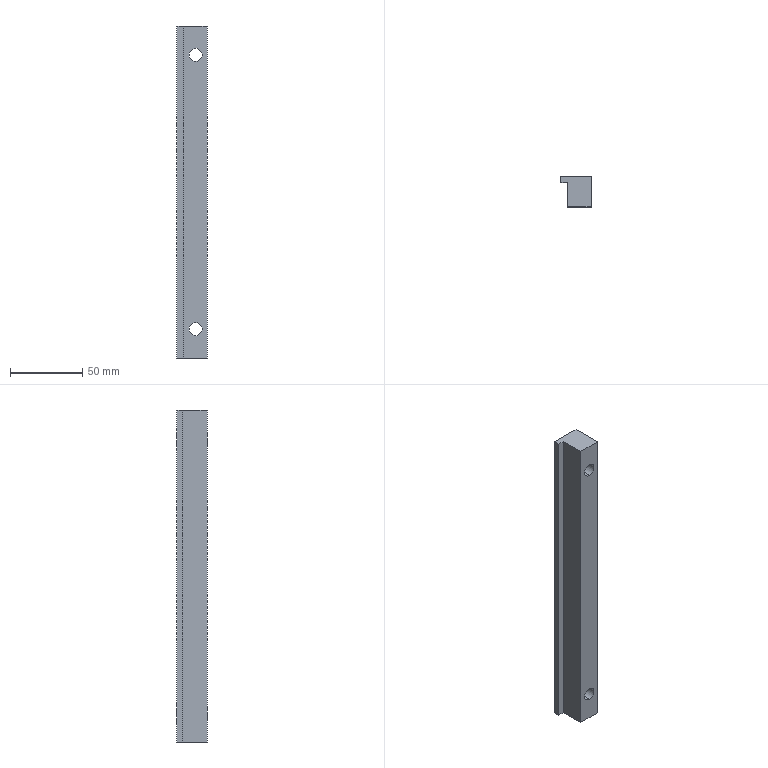Part | STEP file | LM-05-1197_default | 1 solid | 18 faces | box 21 x 21 x 230 mm | volume 79008 mm3 | plane 10 | cylinder 8 | commonest cylinder face diameters 9 x4 15 x4
STEP:
#1=CARTESIAN_POINT('',(0.,0.,0.));
#2=DIRECTION('',(0.,0.,1.));
#3=DIRECTION('',(1.,0.,0.));
#4=AXIS2_PLACEMENT_3D('',#1,#2,#3);
#5=CARTESIAN_POINT('',(13.,-8.6,217.5));
#6=VERTEX_POINT('',#5);
#7=CARTESIAN_POINT('',(13.,0.,217.5));
#8=VERTEX_POINT('',#7);
#9=CARTESIAN_POINT('',(13.,0.,217.5));
#10=DIRECTION('',(0.,1.,0.));
#11=VECTOR('',#10,1.);
#12=LINE('',#9,#11);
#13=CARTESIAN_POINT('',(13.,0.,210.));
#14=DIRECTION('',(0.,1.,0.));
#15=DIRECTION('',(0.,0.,1.));
#16=AXIS2_PLACEMENT_3D('',#13,#14,#15);
#17=CYLINDRICAL_SURFACE('',#16,7.5);
#18=CARTESIAN_POINT('',(6.283,0.));
#19=DIRECTION('',(0.,1.));
#20=VECTOR('',#19,1.);
#21=LINE('',#18,#20);
#22=(GEOMETRIC_REPRESENTATION_CONTEXT(2)PARAMETRIC_REPRESENTATION_CONTEXT()REPRESENTATION_CONTEXT('',''));
#23=DEFINITIONAL_REPRESENTATION('',(#21),#22);
#24=PCURVE('',#17,#23);
#25=CARTESIAN_POINT('',(13.,0.,210.));
#26=DIRECTION('',(0.,1.,0.));
#27=DIRECTION('',(0.,0.,1.));
#28=AXIS2_PLACEMENT_3D('',#25,#26,#27);
#29=CYLINDRICAL_SURFACE('',#28,7.5);
#30=CARTESIAN_POINT('',(0.,0.));
#31=DIRECTION('',(0.,1.));
#32=VECTOR('',#31,1.);
#33=LINE('',#30,#32);
#34=(GEOMETRIC_REPRESENTATION_CONTEXT(2)PARAMETRIC_REPRESENTATION_CONTEXT()REPRESENTATION_CONTEXT('',''));
#35=DEFINITIONAL_REPRESENTATION('',(#33),#34);
#36=PCURVE('',#29,#35);
#37=SURFACE_CURVE('',#12,(#24,#36),.PCURVE_S1.);
#38=EDGE_CURVE('',#6,#8,#37,.T.);
#39=ORIENTED_EDGE('',*,*,#38,.T.);
#40=CARTESIAN_POINT('',(13.,0.,202.5));
#41=VERTEX_POINT('',#40);
#42=CARTESIAN_POINT('',(13.,0.,210.));
#43=DIRECTION('',(0.,1.,0.));
#44=DIRECTION('',(0.,0.,1.));
#45=AXIS2_PLACEMENT_3D('',#42,#43,#44);
#46=CIRCLE('',#45,7.5);
#47=CARTESIAN_POINT('',(0.,0.));
#48=DIRECTION('',(1.,0.));
#49=VECTOR('',#48,1.);
#50=LINE('',#47,#49);
#51=(GEOMETRIC_REPRESENTATION_CONTEXT(2)PARAMETRIC_REPRESENTATION_CONTEXT()REPRESENTATION_CONTEXT('',''));
#52=DEFINITIONAL_REPRESENTATION('',(#50),#51);
#53=PCURVE('',#17,#52);
#54=CARTESIAN_POINT('',(21.,0.,230.));
#55=DIRECTION('',(0.,-1.,0.));
#56=DIRECTION('',(1.,0.,0.));
#57=AXIS2_PLACEMENT_3D('',#54,#55,#56);
#58=PLANE('',#57);
#59=CARTESIAN_POINT('',(-8.,-12.5));
#60=CARTESIAN_POINT('',(4.99,-12.5));
#61=CARTESIAN_POINT('',(-1.505,-23.75));
#62=CARTESIAN_POINT('',(-8.,-35.));
#63=CARTESIAN_POINT('',(-14.495,-23.75));
#64=CARTESIAN_POINT('',(-20.99,-12.5));
#65=CARTESIAN_POINT('',(-8.,-12.5));
#66=(BOUNDED_CURVE()B_SPLINE_CURVE(2,(#59,#60,#61,#62,#63,#64,#65),.UNSPECIFIED.,.T.,.F.)B_SPLINE_CURVE_WITH_KNOTS((1,2,2,2,2,1),(-2.094,0.,2.094,4.189,6.283,8.378),.UNSPECIFIED.)CURVE()GEOMETRIC_REPRESENTATION_ITEM()RATIONAL_B_SPLINE_CURVE((1.,0.5,1.,0.5,1.,0.5,1.))REPRESENTATION_ITEM(''));
#67=(GEOMETRIC_REPRESENTATION_CONTEXT(2)PARAMETRIC_REPRESENTATION_CONTEXT()REPRESENTATION_CONTEXT('',''));
#68=DEFINITIONAL_REPRESENTATION('',(#66),#67);
#69=PCURVE('',#58,#68);
#70=SURFACE_CURVE('',#46,(#53,#69),.PCURVE_S1.);
#71=EDGE_CURVE('',#41,#8,#70,.T.);
#72=ORIENTED_EDGE('',*,*,#71,.F.);
#73=CARTESIAN_POINT('',(13.,-8.6,202.5));
#74=VERTEX_POINT('',#73);
#75=CARTESIAN_POINT('',(13.,0.,202.5));
#76=DIRECTION('',(0.,1.,0.));
#77=VECTOR('',#76,1.);
#78=LINE('',#75,#77);
#79=CARTESIAN_POINT('',(3.142,0.));
#80=DIRECTION('',(0.,1.));
#81=VECTOR('',#80,1.);
#82=LINE('',#79,#81);
#83=(GEOMETRIC_REPRESENTATION_CONTEXT(2)PARAMETRIC_REPRESENTATION_CONTEXT()REPRESENTATION_CONTEXT('',''));
#84=DEFINITIONAL_REPRESENTATION('',(#82),#83);
#85=PCURVE('',#17,#84);
#86=CARTESIAN_POINT('',(3.142,0.));
#87=DIRECTION('',(0.,1.));
#88=VECTOR('',#87,1.);
#89=LINE('',#86,#88);
#90=(GEOMETRIC_REPRESENTATION_CONTEXT(2)PARAMETRIC_REPRESENTATION_CONTEXT()REPRESENTATION_CONTEXT('',''));
#91=DEFINITIONAL_REPRESENTATION('',(#89),#90);
#92=PCURVE('',#29,#91);
#93=SURFACE_CURVE('',#78,(#85,#92),.PCURVE_S1.);
#94=EDGE_CURVE('',#74,#41,#93,.T.);
#95=ORIENTED_EDGE('',*,*,#94,.F.);
#96=CARTESIAN_POINT('',(13.,-8.6,210.));
#97=DIRECTION('',(0.,1.,0.));
#98=DIRECTION('',(0.,0.,1.));
#99=AXIS2_PLACEMENT_3D('',#96,#97,#98);
#100=CIRCLE('',#99,7.5);
#101=CARTESIAN_POINT('',(0.,-8.6));
#102=DIRECTION('',(1.,0.));
#103=VECTOR('',#102,1.);
#104=LINE('',#101,#103);
#105=(GEOMETRIC_REPRESENTATION_CONTEXT(2)PARAMETRIC_REPRESENTATION_CONTEXT()REPRESENTATION_CONTEXT('',''));
#106=DEFINITIONAL_REPRESENTATION('',(#104),#105);
#107=PCURVE('',#17,#106);
#108=CARTESIAN_POINT('',(17.5,-8.6,210.));
#109=DIRECTION('',(0.,-1.,0.));
#110=DIRECTION('',(0.,0.,-1.));
#111=AXIS2_PLACEMENT_3D('',#108,#109,#110);
#112=PLANE('',#111);
#113=CARTESIAN_POINT('',(-7.5,-4.5));
#114=CARTESIAN_POINT('',(-7.5,8.49));
#115=CARTESIAN_POINT('',(3.75,1.995));
#116=CARTESIAN_POINT('',(15.,-4.5));
#117=CARTESIAN_POINT('',(3.75,-10.995));
#118=CARTESIAN_POINT('',(-7.5,-17.49));
#119=CARTESIAN_POINT('',(-7.5,-4.5));
#120=(BOUNDED_CURVE()B_SPLINE_CURVE(2,(#113,#114,#115,#116,#117,#118,#119),.UNSPECIFIED.,.T.,.F.)B_SPLINE_CURVE_WITH_KNOTS((1,2,2,2,2,1),(-2.094,0.,2.094,4.189,6.283,8.378),.UNSPECIFIED.)CURVE()GEOMETRIC_REPRESENTATION_ITEM()RATIONAL_B_SPLINE_CURVE((1.,0.5,1.,0.5,1.,0.5,1.))REPRESENTATION_ITEM(''));
#121=(GEOMETRIC_REPRESENTATION_CONTEXT(2)PARAMETRIC_REPRESENTATION_CONTEXT()REPRESENTATION_CONTEXT('',''));
#122=DEFINITIONAL_REPRESENTATION('',(#120),#121);
#123=PCURVE('',#112,#122);
#124=SURFACE_CURVE('',#100,(#107,#123),.PCURVE_S1.);
#125=EDGE_CURVE('',#74,#6,#124,.T.);
#126=ORIENTED_EDGE('',*,*,#125,.T.);
#127=EDGE_LOOP('',(#39,#72,#95,#126));
#128=FACE_BOUND('',#127,.F.);
#129=ADVANCED_FACE('',(#128),#17,.F.);
#130=CARTESIAN_POINT('',(13.,-21.,214.5));
#131=VERTEX_POINT('',#130);
#132=CARTESIAN_POINT('',(13.,-8.6,214.5));
#133=VERTEX_POINT('',#132);
#134=CARTESIAN_POINT('',(13.,0.,214.5));
#135=DIRECTION('',(0.,1.,0.));
#136=VECTOR('',#135,1.);
#137=LINE('',#134,#136);
#138=CARTESIAN_POINT('',(13.,0.,210.));
#139=DIRECTION('',(0.,1.,0.));
#140=DIRECTION('',(0.,0.,1.));
#141=AXIS2_PLACEMENT_3D('',#138,#139,#140);
#142=CYLINDRICAL_SURFACE('',#141,4.5);
#143=CARTESIAN_POINT('',(6.283,0.));
#144=DIRECTION('',(0.,1.));
#145=VECTOR('',#144,1.);
#146=LINE('',#143,#145);
#147=(GEOMETRIC_REPRESENTATION_CONTEXT(2)PARAMETRIC_REPRESENTATION_CONTEXT()REPRESENTATION_CONTEXT('',''));
#148=DEFINITIONAL_REPRESENTATION('',(#146),#147);
#149=PCURVE('',#142,#148);
#150=CARTESIAN_POINT('',(13.,0.,210.));
#151=DIRECTION('',(0.,1.,0.));
#152=DIRECTION('',(0.,0.,1.));
#153=AXIS2_PLACEMENT_3D('',#150,#151,#152);
#154=CYLINDRICAL_SURFACE('',#153,4.5);
#155=CARTESIAN_POINT('',(0.,0.));
#156=DIRECTION('',(0.,1.));
#157=VECTOR('',#156,1.);
#158=LINE('',#155,#157);
#159=(GEOMETRIC_REPRESENTATION_CONTEXT(2)PARAMETRIC_REPRESENTATION_CONTEXT()REPRESENTATION_CONTEXT('',''));
#160=DEFINITIONAL_REPRESENTATION('',(#158),#159);
#161=PCURVE('',#154,#160);
#162=SURFACE_CURVE('',#137,(#149,#161),.PCURVE_S1.);
#163=EDGE_CURVE('',#131,#133,#162,.T.);
#164=ORIENTED_EDGE('',*,*,#163,.T.);
#165=CARTESIAN_POINT('',(13.,-8.6,205.5));
#166=VERTEX_POINT('',#165);
#167=CARTESIAN_POINT('',(13.,-8.6,210.));
#168=DIRECTION('',(0.,1.,0.));
#169=DIRECTION('',(0.,0.,1.));
#170=AXIS2_PLACEMENT_3D('',#167,#168,#169);
#171=CIRCLE('',#170,4.5);
#172=CARTESIAN_POINT('',(0.,-8.6));
#173=DIRECTION('',(1.,0.));
#174=VECTOR('',#173,1.);
#175=LINE('',#172,#174);
#176=(GEOMETRIC_REPRESENTATION_CONTEXT(2)PARAMETRIC_REPRESENTATION_CONTEXT()REPRESENTATION_CONTEXT('',''));
#177=DEFINITIONAL_REPRESENTATION('',(#175),#176);
#178=PCURVE('',#142,#177);
#179=CARTESIAN_POINT('',(-4.5,-4.5));
#180=CARTESIAN_POINT('',(-4.5,3.294));
#181=CARTESIAN_POINT('',(2.25,-0.6029));
#182=CARTESIAN_POINT('',(9.,-4.5));
#183=CARTESIAN_POINT('',(2.25,-8.397));
#184=CARTESIAN_POINT('',(-4.5,-12.294));
#185=CARTESIAN_POINT('',(-4.5,-4.5));
#186=(BOUNDED_CURVE()B_SPLINE_CURVE(2,(#179,#180,#181,#182,#183,#184,#185),.UNSPECIFIED.,.T.,.F.)B_SPLINE_CURVE_WITH_KNOTS((1,2,2,2,2,1),(-2.094,0.,2.094,4.189,6.283,8.378),.UNSPECIFIED.)CURVE()GEOMETRIC_REPRESENTATION_ITEM()RATIONAL_B_SPLINE_CURVE((1.,0.5,1.,0.5,1.,0.5,1.))REPRESENTATION_ITEM(''));
#187=(GEOMETRIC_REPRESENTATION_CONTEXT(2)PARAMETRIC_REPRESENTATION_CONTEXT()REPRESENTATION_CONTEXT('',''));
#188=DEFINITIONAL_REPRESENTATION('',(#186),#187);
#189=PCURVE('',#112,#188);
#190=SURFACE_CURVE('',#171,(#178,#189),.PCURVE_S1.);
#191=EDGE_CURVE('',#166,#133,#190,.T.);
#192=ORIENTED_EDGE('',*,*,#191,.F.);
#193=CARTESIAN_POINT('',(13.,-21.,205.5));
#194=VERTEX_POINT('',#193);
#195=CARTESIAN_POINT('',(13.,0.,205.5));
#196=DIRECTION('',(0.,1.,0.));
#197=VECTOR('',#196,1.);
#198=LINE('',#195,#197);
#199=CARTESIAN_POINT('',(3.142,0.));
#200=DIRECTION('',(0.,1.));
#201=VECTOR('',#200,1.);
#202=LINE('',#199,#201);
#203=(GEOMETRIC_REPRESENTATION_CONTEXT(2)PARAMETRIC_REPRESENTATION_CONTEXT()REPRESENTATION_CONTEXT('',''));
#204=DEFINITIONAL_REPRESENTATION('',(#202),#203);
#205=PCURVE('',#142,#204);
#206=CARTESIAN_POINT('',(3.142,0.));
#207=DIRECTION('',(0.,1.));
#208=VECTOR('',#207,1.);
#209=LINE('',#206,#208);
#210=(GEOMETRIC_REPRESENTATION_CONTEXT(2)PARAMETRIC_REPRESENTATION_CONTEXT()REPRESENTATION_CONTEXT('',''));
#211=DEFINITIONAL_REPRESENTATION('',(#209),#210);
#212=PCURVE('',#154,#211);
#213=SURFACE_CURVE('',#198,(#205,#212),.PCURVE_S1.);
#214=EDGE_CURVE('',#194,#166,#213,.T.);
#215=ORIENTED_EDGE('',*,*,#214,.F.);
#216=CARTESIAN_POINT('',(13.,-21.,210.));
#217=DIRECTION('',(0.,1.,0.));
#218=DIRECTION('',(0.,0.,1.));
#219=AXIS2_PLACEMENT_3D('',#216,#217,#218);
#220=CIRCLE('',#219,4.5);
#221=CARTESIAN_POINT('',(0.,-21.));
#222=DIRECTION('',(1.,0.));
#223=VECTOR('',#222,1.);
#224=LINE('',#221,#223);
#225=(GEOMETRIC_REPRESENTATION_CONTEXT(2)PARAMETRIC_REPRESENTATION_CONTEXT()REPRESENTATION_CONTEXT('',''));
#226=DEFINITIONAL_REPRESENTATION('',(#224),#225);
#227=PCURVE('',#142,#226);
#228=CARTESIAN_POINT('',(4.554,-21.,230.));
#229=DIRECTION('',(0.,1.,0.));
#230=DIRECTION('',(0.,0.,1.));
#231=AXIS2_PLACEMENT_3D('',#228,#229,#230);
#232=PLANE('',#231);
#233=CARTESIAN_POINT('',(-20.,8.446));
#234=DIRECTION('',(1.,0.));
#235=AXIS2_PLACEMENT_2D('',#233,#234);
#236=CIRCLE('',#235,4.5);
#237=(GEOMETRIC_REPRESENTATION_CONTEXT(2)PARAMETRIC_REPRESENTATION_CONTEXT()REPRESENTATION_CONTEXT('',''));
#238=DEFINITIONAL_REPRESENTATION('',(#236),#237);
#239=PCURVE('',#232,#238);
#240=SURFACE_CURVE('',#220,(#227,#239),.PCURVE_S1.);
#241=EDGE_CURVE('',#194,#131,#240,.T.);
#242=ORIENTED_EDGE('',*,*,#241,.T.);
#243=EDGE_LOOP('',(#164,#192,#215,#242));
#244=FACE_BOUND('',#243,.F.);
#245=ADVANCED_FACE('',(#244),#142,.F.);
#246=CARTESIAN_POINT('',(13.,-8.6,27.5));
#247=VERTEX_POINT('',#246);
#248=CARTESIAN_POINT('',(13.,0.,27.5));
#249=VERTEX_POINT('',#248);
#250=CARTESIAN_POINT('',(13.,0.,27.5));
#251=DIRECTION('',(0.,1.,0.));
#252=VECTOR('',#251,1.);
#253=LINE('',#250,#252);
#254=CARTESIAN_POINT('',(13.,0.,20.));
#255=DIRECTION('',(0.,1.,0.));
#256=DIRECTION('',(0.,0.,1.));
#257=AXIS2_PLACEMENT_3D('',#254,#255,#256);
#258=CYLINDRICAL_SURFACE('',#257,7.5);
#259=CARTESIAN_POINT('',(6.283,0.));
#260=DIRECTION('',(0.,1.));
#261=VECTOR('',#260,1.);
#262=LINE('',#259,#261);
#263=(GEOMETRIC_REPRESENTATION_CONTEXT(2)PARAMETRIC_REPRESENTATION_CONTEXT()REPRESENTATION_CONTEXT('',''));
#264=DEFINITIONAL_REPRESENTATION('',(#262),#263);
#265=PCURVE('',#258,#264);
#266=CARTESIAN_POINT('',(13.,0.,20.));
#267=DIRECTION('',(0.,1.,0.));
#268=DIRECTION('',(0.,0.,1.));
#269=AXIS2_PLACEMENT_3D('',#266,#267,#268);
#270=CYLINDRICAL_SURFACE('',#269,7.5);
#271=CARTESIAN_POINT('',(0.,0.));
#272=DIRECTION('',(0.,1.));
#273=VECTOR('',#272,1.);
#274=LINE('',#271,#273);
#275=(GEOMETRIC_REPRESENTATION_CONTEXT(2)PARAMETRIC_REPRESENTATION_CONTEXT()REPRESENTATION_CONTEXT('',''));
#276=DEFINITIONAL_REPRESENTATION('',(#274),#275);
#277=PCURVE('',#270,#276);
#278=SURFACE_CURVE('',#253,(#265,#277),.PCURVE_S1.);
#279=EDGE_CURVE('',#247,#249,#278,.T.);
#280=ORIENTED_EDGE('',*,*,#279,.T.);
#281=CARTESIAN_POINT('',(13.,0.,12.5));
#282=VERTEX_POINT('',#281);
#283=CARTESIAN_POINT('',(13.,0.,20.));
#284=DIRECTION('',(0.,1.,0.));
#285=DIRECTION('',(0.,0.,1.));
#286=AXIS2_PLACEMENT_3D('',#283,#284,#285);
#287=CIRCLE('',#286,7.5);
#288=CARTESIAN_POINT('',(0.,0.));
#289=DIRECTION('',(1.,0.));
#290=VECTOR('',#289,1.);
#291=LINE('',#288,#290);
#292=(GEOMETRIC_REPRESENTATION_CONTEXT(2)PARAMETRIC_REPRESENTATION_CONTEXT()REPRESENTATION_CONTEXT('',''));
#293=DEFINITIONAL_REPRESENTATION('',(#291),#292);
#294=PCURVE('',#258,#293);
#295=CARTESIAN_POINT('',(-8.,-202.5));
#296=CARTESIAN_POINT('',(4.99,-202.5));
#297=CARTESIAN_POINT('',(-1.505,-213.75));
#298=CARTESIAN_POINT('',(-8.,-225.));
#299=CARTESIAN_POINT('',(-14.495,-213.75));
#300=CARTESIAN_POINT('',(-20.99,-202.5));
#301=CARTESIAN_POINT('',(-8.,-202.5));
#302=(BOUNDED_CURVE()B_SPLINE_CURVE(2,(#295,#296,#297,#298,#299,#300,#301),.UNSPECIFIED.,.T.,.F.)B_SPLINE_CURVE_WITH_KNOTS((1,2,2,2,2,1),(-2.094,0.,2.094,4.189,6.283,8.378),.UNSPECIFIED.)CURVE()GEOMETRIC_REPRESENTATION_ITEM()RATIONAL_B_SPLINE_CURVE((1.,0.5,1.,0.5,1.,0.5,1.))REPRESENTATION_ITEM(''));
#303=(GEOMETRIC_REPRESENTATION_CONTEXT(2)PARAMETRIC_REPRESENTATION_CONTEXT()REPRESENTATION_CONTEXT('',''));
#304=DEFINITIONAL_REPRESENTATION('',(#302),#303);
#305=PCURVE('',#58,#304);
#306=SURFACE_CURVE('',#287,(#294,#305),.PCURVE_S1.);
#307=EDGE_CURVE('',#282,#249,#306,.T.);
#308=ORIENTED_EDGE('',*,*,#307,.F.);
#309=CARTESIAN_POINT('',(13.,-8.6,12.5));
#310=VERTEX_POINT('',#309);
#311=CARTESIAN_POINT('',(13.,0.,12.5));
#312=DIRECTION('',(0.,1.,0.));
#313=VECTOR('',#312,1.);
#314=LINE('',#311,#313);
#315=CARTESIAN_POINT('',(3.142,0.));
#316=DIRECTION('',(0.,1.));
#317=VECTOR('',#316,1.);
#318=LINE('',#315,#317);
#319=(GEOMETRIC_REPRESENTATION_CONTEXT(2)PARAMETRIC_REPRESENTATION_CONTEXT()REPRESENTATION_CONTEXT('',''));
#320=DEFINITIONAL_REPRESENTATION('',(#318),#319);
#321=PCURVE('',#258,#320);
#322=CARTESIAN_POINT('',(3.142,0.));
#323=DIRECTION('',(0.,1.));
#324=VECTOR('',#323,1.);
#325=LINE('',#322,#324);
#326=(GEOMETRIC_REPRESENTATION_CONTEXT(2)PARAMETRIC_REPRESENTATION_CONTEXT()REPRESENTATION_CONTEXT('',''));
#327=DEFINITIONAL_REPRESENTATION('',(#325),#326);
#328=PCURVE('',#270,#327);
#329=SURFACE_CURVE('',#314,(#321,#328),.PCURVE_S1.);
#330=EDGE_CURVE('',#310,#282,#329,.T.);
#331=ORIENTED_EDGE('',*,*,#330,.F.);
#332=CARTESIAN_POINT('',(13.,-8.6,20.));
#333=DIRECTION('',(0.,1.,0.));
#334=DIRECTION('',(0.,0.,1.));
#335=AXIS2_PLACEMENT_3D('',#332,#333,#334);
#336=CIRCLE('',#335,7.5);
#337=CARTESIAN_POINT('',(0.,-8.6));
#338=DIRECTION('',(1.,0.));
#339=VECTOR('',#338,1.);
#340=LINE('',#337,#339);
#341=(GEOMETRIC_REPRESENTATION_CONTEXT(2)PARAMETRIC_REPRESENTATION_CONTEXT()REPRESENTATION_CONTEXT('',''));
#342=DEFINITIONAL_REPRESENTATION('',(#340),#341);
#343=PCURVE('',#258,#342);
#344=CARTESIAN_POINT('',(17.5,-8.6,20.));
#345=DIRECTION('',(0.,-1.,0.));
#346=DIRECTION('',(0.,0.,-1.));
#347=AXIS2_PLACEMENT_3D('',#344,#345,#346);
#348=PLANE('',#347);
#349=CARTESIAN_POINT('',(-7.5,-4.5));
#350=CARTESIAN_POINT('',(-7.5,8.49));
#351=CARTESIAN_POINT('',(3.75,1.995));
#352=CARTESIAN_POINT('',(15.,-4.5));
#353=CARTESIAN_POINT('',(3.75,-10.995));
#354=CARTESIAN_POINT('',(-7.5,-17.49));
#355=CARTESIAN_POINT('',(-7.5,-4.5));
#356=(BOUNDED_CURVE()B_SPLINE_CURVE(2,(#349,#350,#351,#352,#353,#354,#355),.UNSPECIFIED.,.T.,.F.)B_SPLINE_CURVE_WITH_KNOTS((1,2,2,2,2,1),(-2.094,0.,2.094,4.189,6.283,8.378),.UNSPECIFIED.)CURVE()GEOMETRIC_REPRESENTATION_ITEM()RATIONAL_B_SPLINE_CURVE((1.,0.5,1.,0.5,1.,0.5,1.))REPRESENTATION_ITEM(''));
#357=(GEOMETRIC_REPRESENTATION_CONTEXT(2)PARAMETRIC_REPRESENTATION_CONTEXT()REPRESENTATION_CONTEXT('',''));
#358=DEFINITIONAL_REPRESENTATION('',(#356),#357);
#359=PCURVE('',#348,#358);
#360=SURFACE_CURVE('',#336,(#343,#359),.PCURVE_S1.);
#361=EDGE_CURVE('',#310,#247,#360,.T.);
#362=ORIENTED_EDGE('',*,*,#361,.T.);
#363=EDGE_LOOP('',(#280,#308,#331,#362));
#364=FACE_BOUND('',#363,.F.);
#365=ADVANCED_FACE('',(#364),#258,.F.);
#366=CARTESIAN_POINT('',(13.,-21.,24.5));
#367=VERTEX_POINT('',#366);
#368=CARTESIAN_POINT('',(13.,-8.6,24.5));
#369=VERTEX_POINT('',#368);
#370=CARTESIAN_POINT('',(13.,0.,24.5));
#371=DIRECTION('',(0.,1.,0.));
#372=VECTOR('',#371,1.);
#373=LINE('',#370,#372);
#374=CARTESIAN_POINT('',(13.,0.,20.));
#375=DIRECTION('',(0.,1.,0.));
#376=DIRECTION('',(0.,0.,1.));
#377=AXIS2_PLACEMENT_3D('',#374,#375,#376);
#378=CYLINDRICAL_SURFACE('',#377,4.5);
#379=CARTESIAN_POINT('',(6.283,0.));
#380=DIRECTION('',(0.,1.));
#381=VECTOR('',#380,1.);
#382=LINE('',#379,#381);
#383=(GEOMETRIC_REPRESENTATION_CONTEXT(2)PARAMETRIC_REPRESENTATION_CONTEXT()REPRESENTATION_CONTEXT('',''));
#384=DEFINITIONAL_REPRESENTATION('',(#382),#383);
#385=PCURVE('',#378,#384);
#386=CARTESIAN_POINT('',(13.,0.,20.));
#387=DIRECTION('',(0.,1.,0.));
#388=DIRECTION('',(0.,0.,1.));
#389=AXIS2_PLACEMENT_3D('',#386,#387,#388);
#390=CYLINDRICAL_SURFACE('',#389,4.5);
#391=CARTESIAN_POINT('',(0.,0.));
#392=DIRECTION('',(0.,1.));
#393=VECTOR('',#392,1.);
#394=LINE('',#391,#393);
#395=(GEOMETRIC_REPRESENTATION_CONTEXT(2)PARAMETRIC_REPRESENTATION_CONTEXT()REPRESENTATION_CONTEXT('',''));
#396=DEFINITIONAL_REPRESENTATION('',(#394),#395);
#397=PCURVE('',#390,#396);
#398=SURFACE_CURVE('',#373,(#385,#397),.PCURVE_S1.);
#399=EDGE_CURVE('',#367,#369,#398,.T.);
#400=ORIENTED_EDGE('',*,*,#399,.T.);
#401=CARTESIAN_POINT('',(13.,-8.6,15.5));
#402=VERTEX_POINT('',#401);
#403=CARTESIAN_POINT('',(13.,-8.6,20.));
#404=DIRECTION('',(0.,1.,0.));
#405=DIRECTION('',(0.,0.,1.));
#406=AXIS2_PLACEMENT_3D('',#403,#404,#405);
#407=CIRCLE('',#406,4.5);
#408=CARTESIAN_POINT('',(0.,-8.6));
#409=DIRECTION('',(1.,0.));
#410=VECTOR('',#409,1.);
#411=LINE('',#408,#410);
#412=(GEOMETRIC_REPRESENTATION_CONTEXT(2)PARAMETRIC_REPRESENTATION_CONTEXT()REPRESENTATION_CONTEXT('',''));
#413=DEFINITIONAL_REPRESENTATION('',(#411),#412);
#414=PCURVE('',#378,#413);
#415=CARTESIAN_POINT('',(-4.5,-4.5));
#416=CARTESIAN_POINT('',(-4.5,3.294));
#417=CARTESIAN_POINT('',(2.25,-0.6029));
#418=CARTESIAN_POINT('',(9.,-4.5));
#419=CARTESIAN_POINT('',(2.25,-8.397));
#420=CARTESIAN_POINT('',(-4.5,-12.294));
#421=CARTESIAN_POINT('',(-4.5,-4.5));
#422=(BOUNDED_CURVE()B_SPLINE_CURVE(2,(#415,#416,#417,#418,#419,#420,#421),.UNSPECIFIED.,.T.,.F.)B_SPLINE_CURVE_WITH_KNOTS((1,2,2,2,2,1),(-2.094,0.,2.094,4.189,6.283,8.378),.UNSPECIFIED.)CURVE()GEOMETRIC_REPRESENTATION_ITEM()RATIONAL_B_SPLINE_CURVE((1.,0.5,1.,0.5,1.,0.5,1.))REPRESENTATION_ITEM(''));
#423=(GEOMETRIC_REPRESENTATION_CONTEXT(2)PARAMETRIC_REPRESENTATION_CONTEXT()REPRESENTATION_CONTEXT('',''));
#424=DEFINITIONAL_REPRESENTATION('',(#422),#423);
#425=PCURVE('',#348,#424);
#426=SURFACE_CURVE('',#407,(#414,#425),.PCURVE_S1.);
#427=EDGE_CURVE('',#402,#369,#426,.T.);
#428=ORIENTED_EDGE('',*,*,#427,.F.);
#429=CARTESIAN_POINT('',(13.,-21.,15.5));
#430=VERTEX_POINT('',#429);
#431=CARTESIAN_POINT('',(13.,0.,15.5));
#432=DIRECTION('',(0.,1.,0.));
#433=VECTOR('',#432,1.);
#434=LINE('',#431,#433);
#435=CARTESIAN_POINT('',(3.142,0.));
#436=DIRECTION('',(0.,1.));
#437=VECTOR('',#436,1.);
#438=LINE('',#435,#437);
#439=(GEOMETRIC_REPRESENTATION_CONTEXT(2)PARAMETRIC_REPRESENTATION_CONTEXT()REPRESENTATION_CONTEXT('',''));
#440=DEFINITIONAL_REPRESENTATION('',(#438),#439);
#441=PCURVE('',#378,#440);
#442=CARTESIAN_POINT('',(3.142,0.));
#443=DIRECTION('',(0.,1.));
#444=VECTOR('',#443,1.);
#445=LINE('',#442,#444);
#446=(GEOMETRIC_REPRESENTATION_CONTEXT(2)PARAMETRIC_REPRESENTATION_CONTEXT()REPRESENTATION_CONTEXT('',''));
#447=DEFINITIONAL_REPRESENTATION('',(#445),#446);
#448=PCURVE('',#390,#447);
#449=SURFACE_CURVE('',#434,(#441,#448),.PCURVE_S1.);
#450=EDGE_CURVE('',#430,#402,#449,.T.);
#451=ORIENTED_EDGE('',*,*,#450,.F.);
#452=CARTESIAN_POINT('',(13.,-21.,20.));
#453=DIRECTION('',(0.,1.,0.));
#454=DIRECTION('',(0.,0.,1.));
#455=AXIS2_PLACEMENT_3D('',#452,#453,#454);
#456=CIRCLE('',#455,4.5);
#457=CARTESIAN_POINT('',(0.,-21.));
#458=DIRECTION('',(1.,0.));
#459=VECTOR('',#458,1.);
#460=LINE('',#457,#459);
#461=(GEOMETRIC_REPRESENTATION_CONTEXT(2)PARAMETRIC_REPRESENTATION_CONTEXT()REPRESENTATION_CONTEXT('',''));
#462=DEFINITIONAL_REPRESENTATION('',(#460),#461);
#463=PCURVE('',#378,#462);
#464=CARTESIAN_POINT('',(-210.,8.446));
#465=DIRECTION('',(1.,0.));
#466=AXIS2_PLACEMENT_2D('',#464,#465);
#467=CIRCLE('',#466,4.5);
#468=(GEOMETRIC_REPRESENTATION_CONTEXT(2)PARAMETRIC_REPRESENTATION_CONTEXT()REPRESENTATION_CONTEXT('',''));
#469=DEFINITIONAL_REPRESENTATION('',(#467),#468);
#470=PCURVE('',#232,#469);
#471=SURFACE_CURVE('',#456,(#463,#470),.PCURVE_S1.);
#472=EDGE_CURVE('',#430,#367,#471,.T.);
#473=ORIENTED_EDGE('',*,*,#472,.T.);
#474=EDGE_LOOP('',(#400,#428,#451,#473));
#475=FACE_BOUND('',#474,.F.);
#476=ADVANCED_FACE('',(#475),#378,.F.);
#477=CARTESIAN_POINT('',(13.,0.,210.));
#478=DIRECTION('',(0.,1.,0.));
#479=DIRECTION('',(0.,0.,1.));
#480=AXIS2_PLACEMENT_3D('',#477,#478,#479);
#481=CIRCLE('',#480,7.5);
#482=CARTESIAN_POINT('',(-8.,-12.5));
#483=CARTESIAN_POINT('',(4.99,-12.5));
#484=CARTESIAN_POINT('',(-1.505,-23.75));
#485=CARTESIAN_POINT('',(-8.,-35.));
#486=CARTESIAN_POINT('',(-14.495,-23.75));
#487=CARTESIAN_POINT('',(-20.99,-12.5));
#488=CARTESIAN_POINT('',(-8.,-12.5));
#489=(BOUNDED_CURVE()B_SPLINE_CURVE(2,(#482,#483,#484,#485,#486,#487,#488),.UNSPECIFIED.,.T.,.F.)B_SPLINE_CURVE_WITH_KNOTS((1,2,2,2,2,1),(-2.094,0.,2.094,4.189,6.283,8.378),.UNSPECIFIED.)CURVE()GEOMETRIC_REPRESENTATION_ITEM()RATIONAL_B_SPLINE_CURVE((1.,0.5,1.,0.5,1.,0.5,1.))REPRESENTATION_ITEM(''));
#490=(GEOMETRIC_REPRESENTATION_CONTEXT(2)PARAMETRIC_REPRESENTATION_CONTEXT()REPRESENTATION_CONTEXT('',''));
#491=DEFINITIONAL_REPRESENTATION('',(#489),#490);
#492=PCURVE('',#58,#491);
#493=CARTESIAN_POINT('',(0.,0.));
#494=DIRECTION('',(1.,0.));
#495=VECTOR('',#494,1.);
#496=LINE('',#493,#495);
#497=(GEOMETRIC_REPRESENTATION_CONTEXT(2)PARAMETRIC_REPRESENTATION_CONTEXT()REPRESENTATION_CONTEXT('',''));
#498=DEFINITIONAL_REPRESENTATION('',(#496),#497);
#499=PCURVE('',#29,#498);
#500=SURFACE_CURVE('',#481,(#492,#499),.PCURVE_S1.);
#501=EDGE_CURVE('',#8,#41,#500,.T.);
#502=ORIENTED_EDGE('',*,*,#501,.F.);
#503=ORIENTED_EDGE('',*,*,#71,.F.);
#504=EDGE_LOOP('',(#502,#503));
#505=FACE_BOUND('',#504,.T.);
#506=CARTESIAN_POINT('',(13.,0.,20.));
#507=DIRECTION('',(0.,1.,0.));
#508=DIRECTION('',(0.,0.,1.));
#509=AXIS2_PLACEMENT_3D('',#506,#507,#508);
#510=CIRCLE('',#509,7.5);
#511=CARTESIAN_POINT('',(-8.,-202.5));
#512=CARTESIAN_POINT('',(4.99,-202.5));
#513=CARTESIAN_POINT('',(-1.505,-213.75));
#514=CARTESIAN_POINT('',(-8.,-225.));
#515=CARTESIAN_POINT('',(-14.495,-213.75));
#516=CARTESIAN_POINT('',(-20.99,-202.5));
#517=CARTESIAN_POINT('',(-8.,-202.5));
#518=(BOUNDED_CURVE()B_SPLINE_CURVE(2,(#511,#512,#513,#514,#515,#516,#517),.UNSPECIFIED.,.T.,.F.)B_SPLINE_CURVE_WITH_KNOTS((1,2,2,2,2,1),(-2.094,0.,2.094,4.189,6.283,8.378),.UNSPECIFIED.)CURVE()GEOMETRIC_REPRESENTATION_ITEM()RATIONAL_B_SPLINE_CURVE((1.,0.5,1.,0.5,1.,0.5,1.))REPRESENTATION_ITEM(''));
#519=(GEOMETRIC_REPRESENTATION_CONTEXT(2)PARAMETRIC_REPRESENTATION_CONTEXT()REPRESENTATION_CONTEXT('',''));
#520=DEFINITIONAL_REPRESENTATION('',(#518),#519);
#521=PCURVE('',#58,#520);
#522=CARTESIAN_POINT('',(0.,0.));
#523=DIRECTION('',(1.,0.));
#524=VECTOR('',#523,1.);
#525=LINE('',#522,#524);
#526=(GEOMETRIC_REPRESENTATION_CONTEXT(2)PARAMETRIC_REPRESENTATION_CONTEXT()REPRESENTATION_CONTEXT('',''));
#527=DEFINITIONAL_REPRESENTATION('',(#525),#526);
#528=PCURVE('',#270,#527);
#529=SURFACE_CURVE('',#510,(#521,#528),.PCURVE_S1.);
#530=EDGE_CURVE('',#249,#282,#529,.T.);
#531=ORIENTED_EDGE('',*,*,#530,.F.);
#532=ORIENTED_EDGE('',*,*,#307,.F.);
#533=EDGE_LOOP('',(#531,#532));
#534=FACE_BOUND('',#533,.T.);
#535=CARTESIAN_POINT('',(21.,0.,0.));
#536=VERTEX_POINT('',#535);
#537=CARTESIAN_POINT('',(0.,0.,0.));
#538=VERTEX_POINT('',#537);
#539=CARTESIAN_POINT('',(21.,0.,0.));
#540=DIRECTION('',(-1.,0.,0.));
#541=VECTOR('',#540,1.);
#542=LINE('',#539,#541);
#543=CARTESIAN_POINT('',(0.,-230.));
#544=DIRECTION('',(-1.,0.));
#545=VECTOR('',#544,1.);
#546=LINE('',#543,#545);
#547=(GEOMETRIC_REPRESENTATION_CONTEXT(2)PARAMETRIC_REPRESENTATION_CONTEXT()REPRESENTATION_CONTEXT('',''));
#548=DEFINITIONAL_REPRESENTATION('',(#546),#547);
#549=PCURVE('',#58,#548);
#550=CARTESIAN_POINT('',(0.,0.,0.));
#551=DIRECTION('',(0.,0.,1.));
#552=DIRECTION('',(1.,0.,0.));
#553=AXIS2_PLACEMENT_3D('',#550,#551,#552);
#554=PLANE('',#553);
#555=CARTESIAN_POINT('',(21.,0.));
#556=DIRECTION('',(-1.,0.));
#557=VECTOR('',#556,1.);
#558=LINE('',#555,#557);
#559=(GEOMETRIC_REPRESENTATION_CONTEXT(2)PARAMETRIC_REPRESENTATION_CONTEXT()REPRESENTATION_CONTEXT('',''));
#560=DEFINITIONAL_REPRESENTATION('',(#558),#559);
#561=PCURVE('',#554,#560);
#562=SURFACE_CURVE('',#542,(#549,#561),.PCURVE_S1.);
#563=EDGE_CURVE('',#536,#538,#562,.T.);
#564=ORIENTED_EDGE('',*,*,#563,.T.);
#565=CARTESIAN_POINT('',(0.,0.,230.));
#566=VERTEX_POINT('',#565);
#567=CARTESIAN_POINT('',(0.,0.,230.));
#568=DIRECTION('',(0.,0.,-1.));
#569=VECTOR('',#568,1.);
#570=LINE('',#567,#569);
#571=CARTESIAN_POINT('',(-21.,0.));
#572=DIRECTION('',(0.,-1.));
#573=VECTOR('',#572,1.);
#574=LINE('',#571,#573);
#575=(GEOMETRIC_REPRESENTATION_CONTEXT(2)PARAMETRIC_REPRESENTATION_CONTEXT()REPRESENTATION_CONTEXT('',''));
#576=DEFINITIONAL_REPRESENTATION('',(#574),#575);
#577=PCURVE('',#58,#576);
#578=CARTESIAN_POINT('',(0.,0.,230.));
#579=DIRECTION('',(1.,0.,0.));
#580=DIRECTION('',(0.,1.,0.));
#581=AXIS2_PLACEMENT_3D('',#578,#579,#580);
#582=PLANE('',#581);
#583=CARTESIAN_POINT('',(0.,0.));
#584=DIRECTION('',(0.,-1.));
#585=VECTOR('',#584,1.);
#586=LINE('',#583,#585);
#587=(GEOMETRIC_REPRESENTATION_CONTEXT(2)PARAMETRIC_REPRESENTATION_CONTEXT()REPRESENTATION_CONTEXT('',''));
#588=DEFINITIONAL_REPRESENTATION('',(#586),#587);
#589=PCURVE('',#582,#588);
#590=SURFACE_CURVE('',#570,(#577,#589),.PCURVE_S1.);
#591=EDGE_CURVE('',#566,#538,#590,.T.);
#592=ORIENTED_EDGE('',*,*,#591,.F.);
#593=CARTESIAN_POINT('',(21.,0.,230.));
#594=VERTEX_POINT('',#593);
#595=CARTESIAN_POINT('',(21.,0.,230.));
#596=DIRECTION('',(-1.,0.,0.));
#597=VECTOR('',#596,1.);
#598=LINE('',#595,#597);
#599=CARTESIAN_POINT('',(0.,0.));
#600=DIRECTION('',(-1.,0.));
#601=VECTOR('',#600,1.);
#602=LINE('',#599,#601);
#603=(GEOMETRIC_REPRESENTATION_CONTEXT(2)PARAMETRIC_REPRESENTATION_CONTEXT()REPRESENTATION_CONTEXT('',''));
#604=DEFINITIONAL_REPRESENTATION('',(#602),#603);
#605=PCURVE('',#58,#604);
#606=CARTESIAN_POINT('',(0.,0.,230.));
#607=DIRECTION('',(0.,0.,1.));
#608=DIRECTION('',(1.,0.,0.));
#609=AXIS2_PLACEMENT_3D('',#606,#607,#608);
#610=PLANE('',#609);
#611=CARTESIAN_POINT('',(21.,0.));
#612=DIRECTION('',(-1.,0.));
#613=VECTOR('',#612,1.);
#614=LINE('',#611,#613);
#615=(GEOMETRIC_REPRESENTATION_CONTEXT(2)PARAMETRIC_REPRESENTATION_CONTEXT()REPRESENTATION_CONTEXT('',''));
#616=DEFINITIONAL_REPRESENTATION('',(#614),#615);
#617=PCURVE('',#610,#616);
#618=SURFACE_CURVE('',#598,(#605,#617),.PCURVE_S1.);
#619=EDGE_CURVE('',#594,#566,#618,.T.);
#620=ORIENTED_EDGE('',*,*,#619,.F.);
#621=CARTESIAN_POINT('',(21.,0.,230.));
#622=DIRECTION('',(0.,0.,-1.));
#623=VECTOR('',#622,1.);
#624=LINE('',#621,#623);
#625=CARTESIAN_POINT('',(0.,0.));
#626=DIRECTION('',(0.,-1.));
#627=VECTOR('',#626,1.);
#628=LINE('',#625,#627);
#629=(GEOMETRIC_REPRESENTATION_CONTEXT(2)PARAMETRIC_REPRESENTATION_CONTEXT()REPRESENTATION_CONTEXT('',''));
#630=DEFINITIONAL_REPRESENTATION('',(#628),#629);
#631=PCURVE('',#58,#630);
#632=CARTESIAN_POINT('',(21.,-21.,230.));
#633=DIRECTION('',(-1.,0.,0.));
#634=DIRECTION('',(0.,0.,1.));
#635=AXIS2_PLACEMENT_3D('',#632,#633,#634);
#636=PLANE('',#635);
#637=CARTESIAN_POINT('',(0.,21.));
#638=DIRECTION('',(-1.,0.));
#639=VECTOR('',#638,1.);
#640=LINE('',#637,#639);
#641=(GEOMETRIC_REPRESENTATION_CONTEXT(2)PARAMETRIC_REPRESENTATION_CONTEXT()REPRESENTATION_CONTEXT('',''));
#642=DEFINITIONAL_REPRESENTATION('',(#640),#641);
#643=PCURVE('',#636,#642);
#644=SURFACE_CURVE('',#624,(#631,#643),.PCURVE_S1.);
#645=EDGE_CURVE('',#594,#536,#644,.T.);
#646=ORIENTED_EDGE('',*,*,#645,.T.);
#647=EDGE_LOOP('',(#564,#592,#620,#646));
#648=FACE_BOUND('',#647,.T.);
#649=ADVANCED_FACE('',(#505,#534,#648),#58,.F.);
#650=CARTESIAN_POINT('',(0.,-4.,0.));
#651=VERTEX_POINT('',#650);
#652=CARTESIAN_POINT('',(0.,0.,0.));
#653=DIRECTION('',(0.,-1.,0.));
#654=VECTOR('',#653,1.);
#655=LINE('',#652,#654);
#656=CARTESIAN_POINT('',(0.,-230.));
#657=DIRECTION('',(-1.,0.));
#658=VECTOR('',#657,1.);
#659=LINE('',#656,#658);
#660=(GEOMETRIC_REPRESENTATION_CONTEXT(2)PARAMETRIC_REPRESENTATION_CONTEXT()REPRESENTATION_CONTEXT('',''));
#661=DEFINITIONAL_REPRESENTATION('',(#659),#660);
#662=PCURVE('',#582,#661);
#663=CARTESIAN_POINT('',(0.,0.));
#664=DIRECTION('',(0.,-1.));
#665=VECTOR('',#664,1.);
#666=LINE('',#663,#665);
#667=(GEOMETRIC_REPRESENTATION_CONTEXT(2)PARAMETRIC_REPRESENTATION_CONTEXT()REPRESENTATION_CONTEXT('',''));
#668=DEFINITIONAL_REPRESENTATION('',(#666),#667);
#669=PCURVE('',#554,#668);
#670=SURFACE_CURVE('',#655,(#662,#669),.PCURVE_S1.);
#671=EDGE_CURVE('',#538,#651,#670,.T.);
#672=ORIENTED_EDGE('',*,*,#671,.T.);
#673=CARTESIAN_POINT('',(0.,-4.,230.));
#674=VERTEX_POINT('',#673);
#675=CARTESIAN_POINT('',(0.,-4.,230.));
#676=DIRECTION('',(0.,0.,-1.));
#677=VECTOR('',#676,1.);
#678=LINE('',#675,#677);
#679=CARTESIAN_POINT('',(-4.,0.));
#680=DIRECTION('',(0.,-1.));
#681=VECTOR('',#680,1.);
#682=LINE('',#679,#681);
#683=(GEOMETRIC_REPRESENTATION_CONTEXT(2)PARAMETRIC_REPRESENTATION_CONTEXT()REPRESENTATION_CONTEXT('',''));
#684=DEFINITIONAL_REPRESENTATION('',(#682),#683);
#685=PCURVE('',#582,#684);
#686=CARTESIAN_POINT('',(0.,-4.,230.));
#687=DIRECTION('',(0.,1.,0.));
#688=DIRECTION('',(0.,0.,1.));
#689=AXIS2_PLACEMENT_3D('',#686,#687,#688);
#690=PLANE('',#689);
#691=CARTESIAN_POINT('',(0.,0.));
#692=DIRECTION('',(-1.,0.));
#693=VECTOR('',#692,1.);
#694=LINE('',#691,#693);
#695=(GEOMETRIC_REPRESENTATION_CONTEXT(2)PARAMETRIC_REPRESENTATION_CONTEXT()REPRESENTATION_CONTEXT('',''));
#696=DEFINITIONAL_REPRESENTATION('',(#694),#695);
#697=PCURVE('',#690,#696);
#698=SURFACE_CURVE('',#678,(#685,#697),.PCURVE_S1.);
#699=EDGE_CURVE('',#674,#651,#698,.T.);
#700=ORIENTED_EDGE('',*,*,#699,.F.);
#701=CARTESIAN_POINT('',(0.,0.,230.));
#702=DIRECTION('',(0.,-1.,0.));
#703=VECTOR('',#702,1.);
#704=LINE('',#701,#703);
#705=CARTESIAN_POINT('',(0.,0.));
#706=DIRECTION('',(-1.,0.));
#707=VECTOR('',#706,1.);
#708=LINE('',#705,#707);
#709=(GEOMETRIC_REPRESENTATION_CONTEXT(2)PARAMETRIC_REPRESENTATION_CONTEXT()REPRESENTATION_CONTEXT('',''));
#710=DEFINITIONAL_REPRESENTATION('',(#708),#709);
#711=PCURVE('',#582,#710);
#712=CARTESIAN_POINT('',(0.,0.));
#713=DIRECTION('',(0.,-1.));
#714=VECTOR('',#713,1.);
#715=LINE('',#712,#714);
#716=(GEOMETRIC_REPRESENTATION_CONTEXT(2)PARAMETRIC_REPRESENTATION_CONTEXT()REPRESENTATION_CONTEXT('',''));
#717=DEFINITIONAL_REPRESENTATION('',(#715),#716);
#718=PCURVE('',#610,#717);
#719=SURFACE_CURVE('',#704,(#711,#718),.PCURVE_S1.);
#720=EDGE_CURVE('',#566,#674,#719,.T.);
#721=ORIENTED_EDGE('',*,*,#720,.F.);
#722=ORIENTED_EDGE('',*,*,#591,.T.);
#723=EDGE_LOOP('',(#672,#700,#721,#722));
#724=FACE_BOUND('',#723,.T.);
#725=ADVANCED_FACE('',(#724),#582,.F.);
#726=CARTESIAN_POINT('',(4.554,-4.,0.));
#727=VERTEX_POINT('',#726);
#728=CARTESIAN_POINT('',(0.,-4.,0.));
#729=DIRECTION('',(1.,0.,0.));
#730=VECTOR('',#729,1.);
#731=LINE('',#728,#730);
#732=CARTESIAN_POINT('',(-230.,0.));
#733=DIRECTION('',(0.,1.));
#734=VECTOR('',#733,1.);
#735=LINE('',#732,#734);
#736=(GEOMETRIC_REPRESENTATION_CONTEXT(2)PARAMETRIC_REPRESENTATION_CONTEXT()REPRESENTATION_CONTEXT('',''));
#737=DEFINITIONAL_REPRESENTATION('',(#735),#736);
#738=PCURVE('',#690,#737);
#739=CARTESIAN_POINT('',(0.,-4.));
#740=DIRECTION('',(1.,0.));
#741=VECTOR('',#740,1.);
#742=LINE('',#739,#741);
#743=(GEOMETRIC_REPRESENTATION_CONTEXT(2)PARAMETRIC_REPRESENTATION_CONTEXT()REPRESENTATION_CONTEXT('',''));
#744=DEFINITIONAL_REPRESENTATION('',(#742),#743);
#745=PCURVE('',#554,#744);
#746=SURFACE_CURVE('',#731,(#738,#745),.PCURVE_S1.);
#747=EDGE_CURVE('',#651,#727,#746,.T.);
#748=ORIENTED_EDGE('',*,*,#747,.T.);
#749=CARTESIAN_POINT('',(4.554,-4.,230.));
#750=VERTEX_POINT('',#749);
#751=CARTESIAN_POINT('',(4.554,-4.,230.));
#752=DIRECTION('',(0.,0.,-1.));
#753=VECTOR('',#752,1.);
#754=LINE('',#751,#753);
#755=CARTESIAN_POINT('',(0.,4.554));
#756=DIRECTION('',(-1.,0.));
#757=VECTOR('',#756,1.);
#758=LINE('',#755,#757);
#759=(GEOMETRIC_REPRESENTATION_CONTEXT(2)PARAMETRIC_REPRESENTATION_CONTEXT()REPRESENTATION_CONTEXT('',''));
#760=DEFINITIONAL_REPRESENTATION('',(#758),#759);
#761=PCURVE('',#690,#760);
#762=CARTESIAN_POINT('',(4.554,-4.,230.));
#763=DIRECTION('',(1.,0.,0.));
#764=DIRECTION('',(0.,1.,0.));
#765=AXIS2_PLACEMENT_3D('',#762,#763,#764);
#766=PLANE('',#765);
#767=CARTESIAN_POINT('',(0.,0.));
#768=DIRECTION('',(0.,-1.));
#769=VECTOR('',#768,1.);
#770=LINE('',#767,#769);
#771=(GEOMETRIC_REPRESENTATION_CONTEXT(2)PARAMETRIC_REPRESENTATION_CONTEXT()REPRESENTATION_CONTEXT('',''));
#772=DEFINITIONAL_REPRESENTATION('',(#770),#771);
#773=PCURVE('',#766,#772);
#774=SURFACE_CURVE('',#754,(#761,#773),.PCURVE_S1.);
#775=EDGE_CURVE('',#750,#727,#774,.T.);
#776=ORIENTED_EDGE('',*,*,#775,.F.);
#777=CARTESIAN_POINT('',(0.,-4.,230.));
#778=DIRECTION('',(1.,0.,0.));
#779=VECTOR('',#778,1.);
#780=LINE('',#777,#779);
#781=CARTESIAN_POINT('',(0.,0.));
#782=DIRECTION('',(0.,1.));
#783=VECTOR('',#782,1.);
#784=LINE('',#781,#783);
#785=(GEOMETRIC_REPRESENTATION_CONTEXT(2)PARAMETRIC_REPRESENTATION_CONTEXT()REPRESENTATION_CONTEXT('',''));
#786=DEFINITIONAL_REPRESENTATION('',(#784),#785);
#787=PCURVE('',#690,#786);
#788=CARTESIAN_POINT('',(0.,-4.));
#789=DIRECTION('',(1.,0.));
#790=VECTOR('',#789,1.);
#791=LINE('',#788,#790);
#792=(GEOMETRIC_REPRESENTATION_CONTEXT(2)PARAMETRIC_REPRESENTATION_CONTEXT()REPRESENTATION_CONTEXT('',''));
#793=DEFINITIONAL_REPRESENTATION('',(#791),#792);
#794=PCURVE('',#610,#793);
#795=SURFACE_CURVE('',#780,(#787,#794),.PCURVE_S1.);
#796=EDGE_CURVE('',#674,#750,#795,.T.);
#797=ORIENTED_EDGE('',*,*,#796,.F.);
#798=ORIENTED_EDGE('',*,*,#699,.T.);
#799=EDGE_LOOP('',(#748,#776,#797,#798));
#800=FACE_BOUND('',#799,.T.);
#801=ADVANCED_FACE('',(#800),#690,.F.);
#802=CARTESIAN_POINT('',(4.554,-21.,0.));
#803=VERTEX_POINT('',#802);
#804=CARTESIAN_POINT('',(4.554,-4.,0.));
#805=DIRECTION('',(0.,-1.,0.));
#806=VECTOR('',#805,1.);
#807=LINE('',#804,#806);
#808=CARTESIAN_POINT('',(0.,-230.));
#809=DIRECTION('',(-1.,0.));
#810=VECTOR('',#809,1.);
#811=LINE('',#808,#810);
#812=(GEOMETRIC_REPRESENTATION_CONTEXT(2)PARAMETRIC_REPRESENTATION_CONTEXT()REPRESENTATION_CONTEXT('',''));
#813=DEFINITIONAL_REPRESENTATION('',(#811),#812);
#814=PCURVE('',#766,#813);
#815=CARTESIAN_POINT('',(4.554,-4.));
#816=DIRECTION('',(0.,-1.));
#817=VECTOR('',#816,1.);
#818=LINE('',#815,#817);
#819=(GEOMETRIC_REPRESENTATION_CONTEXT(2)PARAMETRIC_REPRESENTATION_CONTEXT()REPRESENTATION_CONTEXT('',''));
#820=DEFINITIONAL_REPRESENTATION('',(#818),#819);
#821=PCURVE('',#554,#820);
#822=SURFACE_CURVE('',#807,(#814,#821),.PCURVE_S1.);
#823=EDGE_CURVE('',#727,#803,#822,.T.);
#824=ORIENTED_EDGE('',*,*,#823,.T.);
#825=CARTESIAN_POINT('',(4.554,-21.,230.));
#826=VERTEX_POINT('',#825);
#827=CARTESIAN_POINT('',(4.554,-21.,230.));
#828=DIRECTION('',(0.,0.,-1.));
#829=VECTOR('',#828,1.);
#830=LINE('',#827,#829);
#831=CARTESIAN_POINT('',(-17.,0.));
#832=DIRECTION('',(0.,-1.));
#833=VECTOR('',#832,1.);
#834=LINE('',#831,#833);
#835=(GEOMETRIC_REPRESENTATION_CONTEXT(2)PARAMETRIC_REPRESENTATION_CONTEXT()REPRESENTATION_CONTEXT('',''));
#836=DEFINITIONAL_REPRESENTATION('',(#834),#835);
#837=PCURVE('',#766,#836);
#838=CARTESIAN_POINT('',(0.,0.));
#839=DIRECTION('',(-1.,0.));
#840=VECTOR('',#839,1.);
#841=LINE('',#838,#840);
#842=(GEOMETRIC_REPRESENTATION_CONTEXT(2)PARAMETRIC_REPRESENTATION_CONTEXT()REPRESENTATION_CONTEXT('',''));
#843=DEFINITIONAL_REPRESENTATION('',(#841),#842);
#844=PCURVE('',#232,#843);
#845=SURFACE_CURVE('',#830,(#837,#844),.PCURVE_S1.);
#846=EDGE_CURVE('',#826,#803,#845,.T.);
#847=ORIENTED_EDGE('',*,*,#846,.F.);
#848=CARTESIAN_POINT('',(4.554,-4.,230.));
#849=DIRECTION('',(0.,-1.,0.));
#850=VECTOR('',#849,1.);
#851=LINE('',#848,#850);
#852=CARTESIAN_POINT('',(0.,0.));
#853=DIRECTION('',(-1.,0.));
#854=VECTOR('',#853,1.);
#855=LINE('',#852,#854);
#856=(GEOMETRIC_REPRESENTATION_CONTEXT(2)PARAMETRIC_REPRESENTATION_CONTEXT()REPRESENTATION_CONTEXT('',''));
#857=DEFINITIONAL_REPRESENTATION('',(#855),#856);
#858=PCURVE('',#766,#857);
#859=CARTESIAN_POINT('',(4.554,-4.));
#860=DIRECTION('',(0.,-1.));
#861=VECTOR('',#860,1.);
#862=LINE('',#859,#861);
#863=(GEOMETRIC_REPRESENTATION_CONTEXT(2)PARAMETRIC_REPRESENTATION_CONTEXT()REPRESENTATION_CONTEXT('',''));
#864=DEFINITIONAL_REPRESENTATION('',(#862),#863);
#865=PCURVE('',#610,#864);
#866=SURFACE_CURVE('',#851,(#858,#865),.PCURVE_S1.);
#867=EDGE_CURVE('',#750,#826,#866,.T.);
#868=ORIENTED_EDGE('',*,*,#867,.F.);
#869=ORIENTED_EDGE('',*,*,#775,.T.);
#870=EDGE_LOOP('',(#824,#847,#868,#869));
#871=FACE_BOUND('',#870,.T.);
#872=ADVANCED_FACE('',(#871),#766,.F.);
#873=CARTESIAN_POINT('',(13.,-21.,210.));
#874=DIRECTION('',(0.,1.,0.));
#875=DIRECTION('',(0.,0.,1.));
#876=AXIS2_PLACEMENT_3D('',#873,#874,#875);
#877=CIRCLE('',#876,4.5);
#878=CARTESIAN_POINT('',(-20.,8.446));
#879=DIRECTION('',(1.,0.));
#880=AXIS2_PLACEMENT_2D('',#878,#879);
#881=CIRCLE('',#880,4.5);
#882=(GEOMETRIC_REPRESENTATION_CONTEXT(2)PARAMETRIC_REPRESENTATION_CONTEXT()REPRESENTATION_CONTEXT('',''));
#883=DEFINITIONAL_REPRESENTATION('',(#881),#882);
#884=PCURVE('',#232,#883);
#885=CARTESIAN_POINT('',(0.,-21.));
#886=DIRECTION('',(1.,0.));
#887=VECTOR('',#886,1.);
#888=LINE('',#885,#887);
#889=(GEOMETRIC_REPRESENTATION_CONTEXT(2)PARAMETRIC_REPRESENTATION_CONTEXT()REPRESENTATION_CONTEXT('',''));
#890=DEFINITIONAL_REPRESENTATION('',(#888),#889);
#891=PCURVE('',#154,#890);
#892=SURFACE_CURVE('',#877,(#884,#891),.PCURVE_S1.);
#893=EDGE_CURVE('',#131,#194,#892,.T.);
#894=ORIENTED_EDGE('',*,*,#893,.T.);
#895=ORIENTED_EDGE('',*,*,#241,.T.);
#896=EDGE_LOOP('',(#894,#895));
#897=FACE_BOUND('',#896,.T.);
#898=CARTESIAN_POINT('',(13.,-21.,20.));
#899=DIRECTION('',(0.,1.,0.));
#900=DIRECTION('',(0.,0.,1.));
#901=AXIS2_PLACEMENT_3D('',#898,#899,#900);
#902=CIRCLE('',#901,4.5);
#903=CARTESIAN_POINT('',(-210.,8.446));
#904=DIRECTION('',(1.,0.));
#905=AXIS2_PLACEMENT_2D('',#903,#904);
#906=CIRCLE('',#905,4.5);
#907=(GEOMETRIC_REPRESENTATION_CONTEXT(2)PARAMETRIC_REPRESENTATION_CONTEXT()REPRESENTATION_CONTEXT('',''));
#908=DEFINITIONAL_REPRESENTATION('',(#906),#907);
#909=PCURVE('',#232,#908);
#910=CARTESIAN_POINT('',(0.,-21.));
#911=DIRECTION('',(1.,0.));
#912=VECTOR('',#911,1.);
#913=LINE('',#910,#912);
#914=(GEOMETRIC_REPRESENTATION_CONTEXT(2)PARAMETRIC_REPRESENTATION_CONTEXT()REPRESENTATION_CONTEXT('',''));
#915=DEFINITIONAL_REPRESENTATION('',(#913),#914);
#916=PCURVE('',#390,#915);
#917=SURFACE_CURVE('',#902,(#909,#916),.PCURVE_S1.);
#918=EDGE_CURVE('',#367,#430,#917,.T.);
#919=ORIENTED_EDGE('',*,*,#918,.T.);
#920=ORIENTED_EDGE('',*,*,#472,.T.);
#921=EDGE_LOOP('',(#919,#920));
#922=FACE_BOUND('',#921,.T.);
#923=CARTESIAN_POINT('',(21.,-21.,0.));
#924=VERTEX_POINT('',#923);
#925=CARTESIAN_POINT('',(4.554,-21.,0.));
#926=DIRECTION('',(1.,0.,0.));
#927=VECTOR('',#926,1.);
#928=LINE('',#925,#927);
#929=CARTESIAN_POINT('',(-230.,0.));
#930=DIRECTION('',(0.,1.));
#931=VECTOR('',#930,1.);
#932=LINE('',#929,#931);
#933=(GEOMETRIC_REPRESENTATION_CONTEXT(2)PARAMETRIC_REPRESENTATION_CONTEXT()REPRESENTATION_CONTEXT('',''));
#934=DEFINITIONAL_REPRESENTATION('',(#932),#933);
#935=PCURVE('',#232,#934);
#936=CARTESIAN_POINT('',(4.554,-21.));
#937=DIRECTION('',(1.,0.));
#938=VECTOR('',#937,1.);
#939=LINE('',#936,#938);
#940=(GEOMETRIC_REPRESENTATION_CONTEXT(2)PARAMETRIC_REPRESENTATION_CONTEXT()REPRESENTATION_CONTEXT('',''));
#941=DEFINITIONAL_REPRESENTATION('',(#939),#940);
#942=PCURVE('',#554,#941);
#943=SURFACE_CURVE('',#928,(#935,#942),.PCURVE_S1.);
#944=EDGE_CURVE('',#803,#924,#943,.T.);
#945=ORIENTED_EDGE('',*,*,#944,.T.);
#946=CARTESIAN_POINT('',(21.,-21.,230.));
#947=VERTEX_POINT('',#946);
#948=CARTESIAN_POINT('',(21.,-21.,230.));
#949=DIRECTION('',(0.,0.,-1.));
#950=VECTOR('',#949,1.);
#951=LINE('',#948,#950);
#952=CARTESIAN_POINT('',(0.,16.446));
#953=DIRECTION('',(-1.,0.));
#954=VECTOR('',#953,1.);
#955=LINE('',#952,#954);
#956=(GEOMETRIC_REPRESENTATION_CONTEXT(2)PARAMETRIC_REPRESENTATION_CONTEXT()REPRESENTATION_CONTEXT('',''));
#957=DEFINITIONAL_REPRESENTATION('',(#955),#956);
#958=PCURVE('',#232,#957);
#959=CARTESIAN_POINT('',(0.,0.));
#960=DIRECTION('',(-1.,0.));
#961=VECTOR('',#960,1.);
#962=LINE('',#959,#961);
#963=(GEOMETRIC_REPRESENTATION_CONTEXT(2)PARAMETRIC_REPRESENTATION_CONTEXT()REPRESENTATION_CONTEXT('',''));
#964=DEFINITIONAL_REPRESENTATION('',(#962),#963);
#965=PCURVE('',#636,#964);
#966=SURFACE_CURVE('',#951,(#958,#965),.PCURVE_S1.);
#967=EDGE_CURVE('',#947,#924,#966,.T.);
#968=ORIENTED_EDGE('',*,*,#967,.F.);
#969=CARTESIAN_POINT('',(4.554,-21.,230.));
#970=DIRECTION('',(1.,0.,0.));
#971=VECTOR('',#970,1.);
#972=LINE('',#969,#971);
#973=CARTESIAN_POINT('',(0.,0.));
#974=DIRECTION('',(0.,1.));
#975=VECTOR('',#974,1.);
#976=LINE('',#973,#975);
#977=(GEOMETRIC_REPRESENTATION_CONTEXT(2)PARAMETRIC_REPRESENTATION_CONTEXT()REPRESENTATION_CONTEXT('',''));
#978=DEFINITIONAL_REPRESENTATION('',(#976),#977);
#979=PCURVE('',#232,#978);
#980=CARTESIAN_POINT('',(4.554,-21.));
#981=DIRECTION('',(1.,0.));
#982=VECTOR('',#981,1.);
#983=LINE('',#980,#982);
#984=(GEOMETRIC_REPRESENTATION_CONTEXT(2)PARAMETRIC_REPRESENTATION_CONTEXT()REPRESENTATION_CONTEXT('',''));
#985=DEFINITIONAL_REPRESENTATION('',(#983),#984);
#986=PCURVE('',#610,#985);
#987=SURFACE_CURVE('',#972,(#979,#986),.PCURVE_S1.);
#988=EDGE_CURVE('',#826,#947,#987,.T.);
#989=ORIENTED_EDGE('',*,*,#988,.F.);
#990=ORIENTED_EDGE('',*,*,#846,.T.);
#991=EDGE_LOOP('',(#945,#968,#989,#990));
#992=FACE_BOUND('',#991,.T.);
#993=ADVANCED_FACE('',(#897,#922,#992),#232,.F.);
#994=CARTESIAN_POINT('',(21.,-21.,0.));
#995=DIRECTION('',(0.,1.,0.));
#996=VECTOR('',#995,1.);
#997=LINE('',#994,#996);
#998=CARTESIAN_POINT('',(-230.,0.));
#999=DIRECTION('',(0.,1.));
#1000=VECTOR('',#999,1.);
#1001=LINE('',#998,#1000);
#1002=(GEOMETRIC_REPRESENTATION_CONTEXT(2)PARAMETRIC_REPRESENTATION_CONTEXT()REPRESENTATION_CONTEXT('',''));
#1003=DEFINITIONAL_REPRESENTATION('',(#1001),#1002);
#1004=PCURVE('',#636,#1003);
#1005=CARTESIAN_POINT('',(21.,-21.));
#1006=DIRECTION('',(0.,1.));
#1007=VECTOR('',#1006,1.);
#1008=LINE('',#1005,#1007);
#1009=(GEOMETRIC_REPRESENTATION_CONTEXT(2)PARAMETRIC_REPRESENTATION_CONTEXT()REPRESENTATION_CONTEXT('',''));
#1010=DEFINITIONAL_REPRESENTATION('',(#1008),#1009);
#1011=PCURVE('',#554,#1010);
#1012=SURFACE_CURVE('',#997,(#1004,#1011),.PCURVE_S1.);
#1013=EDGE_CURVE('',#924,#536,#1012,.T.);
#1014=ORIENTED_EDGE('',*,*,#1013,.T.);
#1015=ORIENTED_EDGE('',*,*,#645,.F.);
#1016=CARTESIAN_POINT('',(21.,-21.,230.));
#1017=DIRECTION('',(0.,1.,0.));
#1018=VECTOR('',#1017,1.);
#1019=LINE('',#1016,#1018);
#1020=CARTESIAN_POINT('',(0.,0.));
#1021=DIRECTION('',(0.,1.));
#1022=VECTOR('',#1021,1.);
#1023=LINE('',#1020,#1022);
#1024=(GEOMETRIC_REPRESENTATION_CONTEXT(2)PARAMETRIC_REPRESENTATION_CONTEXT()REPRESENTATION_CONTEXT('',''));
#1025=DEFINITIONAL_REPRESENTATION('',(#1023),#1024);
#1026=PCURVE('',#636,#1025);
#1027=CARTESIAN_POINT('',(21.,-21.));
#1028=DIRECTION('',(0.,1.));
#1029=VECTOR('',#1028,1.);
#1030=LINE('',#1027,#1029);
#1031=(GEOMETRIC_REPRESENTATION_CONTEXT(2)PARAMETRIC_REPRESENTATION_CONTEXT()REPRESENTATION_CONTEXT('',''));
#1032=DEFINITIONAL_REPRESENTATION('',(#1030),#1031);
#1033=PCURVE('',#610,#1032);
#1034=SURFACE_CURVE('',#1019,(#1026,#1033),.PCURVE_S1.);
#1035=EDGE_CURVE('',#947,#594,#1034,.T.);
#1036=ORIENTED_EDGE('',*,*,#1035,.F.);
#1037=ORIENTED_EDGE('',*,*,#967,.T.);
#1038=EDGE_LOOP('',(#1014,#1015,#1036,#1037));
#1039=FACE_BOUND('',#1038,.T.);
#1040=ADVANCED_FACE('',(#1039),#636,.F.);
#1041=ORIENTED_EDGE('',*,*,#619,.T.);
#1042=ORIENTED_EDGE('',*,*,#720,.T.);
#1043=ORIENTED_EDGE('',*,*,#796,.T.);
#1044=ORIENTED_EDGE('',*,*,#867,.T.);
#1045=ORIENTED_EDGE('',*,*,#988,.T.);
#1046=ORIENTED_EDGE('',*,*,#1035,.T.);
#1047=EDGE_LOOP('',(#1041,#1042,#1043,#1044,#1045,#1046));
#1048=FACE_BOUND('',#1047,.T.);
#1049=ADVANCED_FACE('',(#1048),#610,.T.);
#1050=ORIENTED_EDGE('',*,*,#563,.F.);
#1051=ORIENTED_EDGE('',*,*,#1013,.F.);
#1052=ORIENTED_EDGE('',*,*,#944,.F.);
#1053=ORIENTED_EDGE('',*,*,#823,.F.);
#1054=ORIENTED_EDGE('',*,*,#747,.F.);
#1055=ORIENTED_EDGE('',*,*,#671,.F.);
#1056=EDGE_LOOP('',(#1050,#1051,#1052,#1053,#1054,#1055));
#1057=FACE_BOUND('',#1056,.T.);
#1058=ADVANCED_FACE('',(#1057),#554,.F.);
#1059=CARTESIAN_POINT('',(13.,-8.6,20.));
#1060=DIRECTION('',(0.,1.,0.));
#1061=DIRECTION('',(0.,0.,1.));
#1062=AXIS2_PLACEMENT_3D('',#1059,#1060,#1061);
#1063=CIRCLE('',#1062,4.5);
#1064=CARTESIAN_POINT('',(0.,-8.6));
#1065=DIRECTION('',(1.,0.));
#1066=VECTOR('',#1065,1.);
#1067=LINE('',#1064,#1066);
#1068=(GEOMETRIC_REPRESENTATION_CONTEXT(2)PARAMETRIC_REPRESENTATION_CONTEXT()REPRESENTATION_CONTEXT('',''));
#1069=DEFINITIONAL_REPRESENTATION('',(#1067),#1068);
#1070=PCURVE('',#390,#1069);
#1071=CARTESIAN_POINT('',(-4.5,-4.5));
#1072=CARTESIAN_POINT('',(-4.5,3.294));
#1073=CARTESIAN_POINT('',(2.25,-0.6029));
#1074=CARTESIAN_POINT('',(9.,-4.5));
#1075=CARTESIAN_POINT('',(2.25,-8.397));
#1076=CARTESIAN_POINT('',(-4.5,-12.294));
#1077=CARTESIAN_POINT('',(-4.5,-4.5));
#1078=(BOUNDED_CURVE()B_SPLINE_CURVE(2,(#1071,#1072,#1073,#1074,#1075,#1076,#1077),.UNSPECIFIED.,.T.,.F.)B_SPLINE_CURVE_WITH_KNOTS((1,2,2,2,2,1),(-2.094,0.,2.094,4.189,6.283,8.378),.UNSPECIFIED.)CURVE()GEOMETRIC_REPRESENTATION_ITEM()RATIONAL_B_SPLINE_CURVE((1.,0.5,1.,0.5,1.,0.5,1.))REPRESENTATION_ITEM(''));
#1079=(GEOMETRIC_REPRESENTATION_CONTEXT(2)PARAMETRIC_REPRESENTATION_CONTEXT()REPRESENTATION_CONTEXT('',''));
#1080=DEFINITIONAL_REPRESENTATION('',(#1078),#1079);
#1081=PCURVE('',#348,#1080);
#1082=SURFACE_CURVE('',#1063,(#1070,#1081),.PCURVE_S1.);
#1083=EDGE_CURVE('',#369,#402,#1082,.T.);
#1084=ORIENTED_EDGE('',*,*,#1083,.F.);
#1085=ORIENTED_EDGE('',*,*,#399,.F.);
#1086=ORIENTED_EDGE('',*,*,#918,.T.);
#1087=ORIENTED_EDGE('',*,*,#450,.T.);
#1088=EDGE_LOOP('',(#1084,#1085,#1086,#1087));
#1089=FACE_BOUND('',#1088,.F.);
#1090=ADVANCED_FACE('',(#1089),#390,.F.);
#1091=ORIENTED_EDGE('',*,*,#1083,.F.);
#1092=ORIENTED_EDGE('',*,*,#427,.F.);
#1093=EDGE_LOOP('',(#1091,#1092));
#1094=FACE_BOUND('',#1093,.T.);
#1095=CARTESIAN_POINT('',(13.,-8.6,20.));
#1096=DIRECTION('',(0.,1.,0.));
#1097=DIRECTION('',(0.,0.,1.));
#1098=AXIS2_PLACEMENT_3D('',#1095,#1096,#1097);
#1099=CIRCLE('',#1098,7.5);
#1100=CARTESIAN_POINT('',(-7.5,-4.5));
#1101=CARTESIAN_POINT('',(-7.5,8.49));
#1102=CARTESIAN_POINT('',(3.75,1.995));
#1103=CARTESIAN_POINT('',(15.,-4.5));
#1104=CARTESIAN_POINT('',(3.75,-10.995));
#1105=CARTESIAN_POINT('',(-7.5,-17.49));
#1106=CARTESIAN_POINT('',(-7.5,-4.5));
#1107=(BOUNDED_CURVE()B_SPLINE_CURVE(2,(#1100,#1101,#1102,#1103,#1104,#1105,#1106),.UNSPECIFIED.,.T.,.F.)B_SPLINE_CURVE_WITH_KNOTS((1,2,2,2,2,1),(-2.094,0.,2.094,4.189,6.283,8.378),.UNSPECIFIED.)CURVE()GEOMETRIC_REPRESENTATION_ITEM()RATIONAL_B_SPLINE_CURVE((1.,0.5,1.,0.5,1.,0.5,1.))REPRESENTATION_ITEM(''));
#1108=(GEOMETRIC_REPRESENTATION_CONTEXT(2)PARAMETRIC_REPRESENTATION_CONTEXT()REPRESENTATION_CONTEXT('',''));
#1109=DEFINITIONAL_REPRESENTATION('',(#1107),#1108);
#1110=PCURVE('',#348,#1109);
#1111=CARTESIAN_POINT('',(0.,-8.6));
#1112=DIRECTION('',(1.,0.));
#1113=VECTOR('',#1112,1.);
#1114=LINE('',#1111,#1113);
#1115=(GEOMETRIC_REPRESENTATION_CONTEXT(2)PARAMETRIC_REPRESENTATION_CONTEXT()REPRESENTATION_CONTEXT('',''));
#1116=DEFINITIONAL_REPRESENTATION('',(#1114),#1115);
#1117=PCURVE('',#270,#1116);
#1118=SURFACE_CURVE('',#1099,(#1110,#1117),.PCURVE_S1.);
#1119=EDGE_CURVE('',#247,#310,#1118,.T.);
#1120=ORIENTED_EDGE('',*,*,#1119,.T.);
#1121=ORIENTED_EDGE('',*,*,#361,.T.);
#1122=EDGE_LOOP('',(#1120,#1121));
#1123=FACE_BOUND('',#1122,.T.);
#1124=ADVANCED_FACE('',(#1094,#1123),#348,.F.);
#1125=ORIENTED_EDGE('',*,*,#530,.F.);
#1126=ORIENTED_EDGE('',*,*,#279,.F.);
#1127=ORIENTED_EDGE('',*,*,#1119,.T.);
#1128=ORIENTED_EDGE('',*,*,#330,.T.);
#1129=EDGE_LOOP('',(#1125,#1126,#1127,#1128));
#1130=FACE_BOUND('',#1129,.F.);
#1131=ADVANCED_FACE('',(#1130),#270,.F.);
#1132=CARTESIAN_POINT('',(13.,-8.6,210.));
#1133=DIRECTION('',(0.,1.,0.));
#1134=DIRECTION('',(0.,0.,1.));
#1135=AXIS2_PLACEMENT_3D('',#1132,#1133,#1134);
#1136=CIRCLE('',#1135,4.5);
#1137=CARTESIAN_POINT('',(0.,-8.6));
#1138=DIRECTION('',(1.,0.));
#1139=VECTOR('',#1138,1.);
#1140=LINE('',#1137,#1139);
#1141=(GEOMETRIC_REPRESENTATION_CONTEXT(2)PARAMETRIC_REPRESENTATION_CONTEXT()REPRESENTATION_CONTEXT('',''));
#1142=DEFINITIONAL_REPRESENTATION('',(#1140),#1141);
#1143=PCURVE('',#154,#1142);
#1144=CARTESIAN_POINT('',(-4.5,-4.5));
#1145=CARTESIAN_POINT('',(-4.5,3.294));
#1146=CARTESIAN_POINT('',(2.25,-0.6029));
#1147=CARTESIAN_POINT('',(9.,-4.5));
#1148=CARTESIAN_POINT('',(2.25,-8.397));
#1149=CARTESIAN_POINT('',(-4.5,-12.294));
#1150=CARTESIAN_POINT('',(-4.5,-4.5));
#1151=(BOUNDED_CURVE()B_SPLINE_CURVE(2,(#1144,#1145,#1146,#1147,#1148,#1149,#1150),.UNSPECIFIED.,.T.,.F.)B_SPLINE_CURVE_WITH_KNOTS((1,2,2,2,2,1),(-2.094,0.,2.094,4.189,6.283,8.378),.UNSPECIFIED.)CURVE()GEOMETRIC_REPRESENTATION_ITEM()RATIONAL_B_SPLINE_CURVE((1.,0.5,1.,0.5,1.,0.5,1.))REPRESENTATION_ITEM(''));
#1152=(GEOMETRIC_REPRESENTATION_CONTEXT(2)PARAMETRIC_REPRESENTATION_CONTEXT()REPRESENTATION_CONTEXT('',''));
#1153=DEFINITIONAL_REPRESENTATION('',(#1151),#1152);
#1154=PCURVE('',#112,#1153);
#1155=SURFACE_CURVE('',#1136,(#1143,#1154),.PCURVE_S1.);
#1156=EDGE_CURVE('',#133,#166,#1155,.T.);
#1157=ORIENTED_EDGE('',*,*,#1156,.F.);
#1158=ORIENTED_EDGE('',*,*,#163,.F.);
#1159=ORIENTED_EDGE('',*,*,#893,.T.);
#1160=ORIENTED_EDGE('',*,*,#214,.T.);
#1161=EDGE_LOOP('',(#1157,#1158,#1159,#1160));
#1162=FACE_BOUND('',#1161,.F.);
#1163=ADVANCED_FACE('',(#1162),#154,.F.);
#1164=ORIENTED_EDGE('',*,*,#1156,.F.);
#1165=ORIENTED_EDGE('',*,*,#191,.F.);
#1166=EDGE_LOOP('',(#1164,#1165));
#1167=FACE_BOUND('',#1166,.T.);
#1168=CARTESIAN_POINT('',(13.,-8.6,210.));
#1169=DIRECTION('',(0.,1.,0.));
#1170=DIRECTION('',(0.,0.,1.));
#1171=AXIS2_PLACEMENT_3D('',#1168,#1169,#1170);
#1172=CIRCLE('',#1171,7.5);
#1173=CARTESIAN_POINT('',(-7.5,-4.5));
#1174=CARTESIAN_POINT('',(-7.5,8.49));
#1175=CARTESIAN_POINT('',(3.75,1.995));
#1176=CARTESIAN_POINT('',(15.,-4.5));
#1177=CARTESIAN_POINT('',(3.75,-10.995));
#1178=CARTESIAN_POINT('',(-7.5,-17.49));
#1179=CARTESIAN_POINT('',(-7.5,-4.5));
#1180=(BOUNDED_CURVE()B_SPLINE_CURVE(2,(#1173,#1174,#1175,#1176,#1177,#1178,#1179),.UNSPECIFIED.,.T.,.F.)B_SPLINE_CURVE_WITH_KNOTS((1,2,2,2,2,1),(-2.094,0.,2.094,4.189,6.283,8.378),.UNSPECIFIED.)CURVE()GEOMETRIC_REPRESENTATION_ITEM()RATIONAL_B_SPLINE_CURVE((1.,0.5,1.,0.5,1.,0.5,1.))REPRESENTATION_ITEM(''));
#1181=(GEOMETRIC_REPRESENTATION_CONTEXT(2)PARAMETRIC_REPRESENTATION_CONTEXT()REPRESENTATION_CONTEXT('',''));
#1182=DEFINITIONAL_REPRESENTATION('',(#1180),#1181);
#1183=PCURVE('',#112,#1182);
#1184=CARTESIAN_POINT('',(0.,-8.6));
#1185=DIRECTION('',(1.,0.));
#1186=VECTOR('',#1185,1.);
#1187=LINE('',#1184,#1186);
#1188=(GEOMETRIC_REPRESENTATION_CONTEXT(2)PARAMETRIC_REPRESENTATION_CONTEXT()REPRESENTATION_CONTEXT('',''));
#1189=DEFINITIONAL_REPRESENTATION('',(#1187),#1188);
#1190=PCURVE('',#29,#1189);
#1191=SURFACE_CURVE('',#1172,(#1183,#1190),.PCURVE_S1.);
#1192=EDGE_CURVE('',#6,#74,#1191,.T.);
#1193=ORIENTED_EDGE('',*,*,#1192,.T.);
#1194=ORIENTED_EDGE('',*,*,#125,.T.);
#1195=EDGE_LOOP('',(#1193,#1194));
#1196=FACE_BOUND('',#1195,.T.);
#1197=ADVANCED_FACE('',(#1167,#1196),#112,.F.);
#1198=ORIENTED_EDGE('',*,*,#501,.F.);
#1199=ORIENTED_EDGE('',*,*,#38,.F.);
#1200=ORIENTED_EDGE('',*,*,#1192,.T.);
#1201=ORIENTED_EDGE('',*,*,#94,.T.);
#1202=EDGE_LOOP('',(#1198,#1199,#1200,#1201));
#1203=FACE_BOUND('',#1202,.F.);
#1204=ADVANCED_FACE('',(#1203),#29,.F.);
#1205=CLOSED_SHELL('',(#129,#245,#365,#476,#649,#725,#801,#872,#993,#1040,#1049,#1058,#1090,#1124,#1131,#1163,#1197,#1204));
#1206=MANIFOLD_SOLID_BREP('',#1205);
#1207=(LENGTH_UNIT()NAMED_UNIT(*)SI_UNIT(.MILLI.,.METRE.));
#1208=UNCERTAINTY_MEASURE_WITH_UNIT(LENGTH_MEASURE(0.0000001),#1207,'','');
#1209=(NAMED_UNIT(*)PLANE_ANGLE_UNIT()SI_UNIT($,.RADIAN.));
#1210=(NAMED_UNIT(*)SI_UNIT($,.STERADIAN.)SOLID_ANGLE_UNIT());
#1211=(GEOMETRIC_REPRESENTATION_CONTEXT(3)GLOBAL_UNCERTAINTY_ASSIGNED_CONTEXT((#1208))GLOBAL_UNIT_ASSIGNED_CONTEXT((#1207,#1209,#1210))REPRESENTATION_CONTEXT('',''));
#1212=ADVANCED_BREP_SHAPE_REPRESENTATION('',(#4,#1206),#1211);